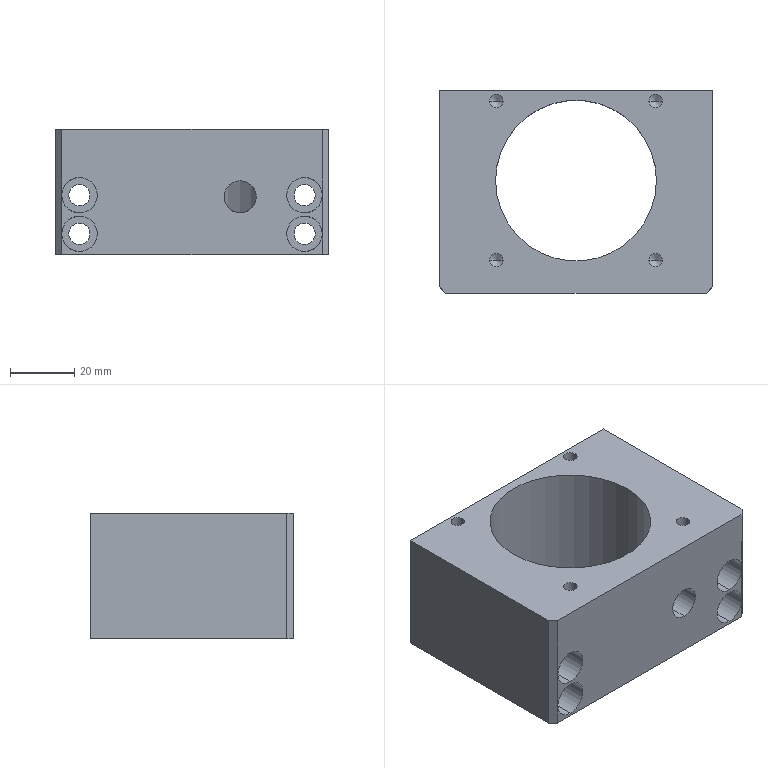Part | SolidWorks | features BaseBody 1 | 1 solid | 57 faces | box 85 x 63 x 39 mm | volume 111586 mm3 | cylinder 32 | plane 15 | cone 10 | commonest cylinder face diameters 4.2 x8 6.6 x8 11 x8 5 x4 10 x2 50 x2